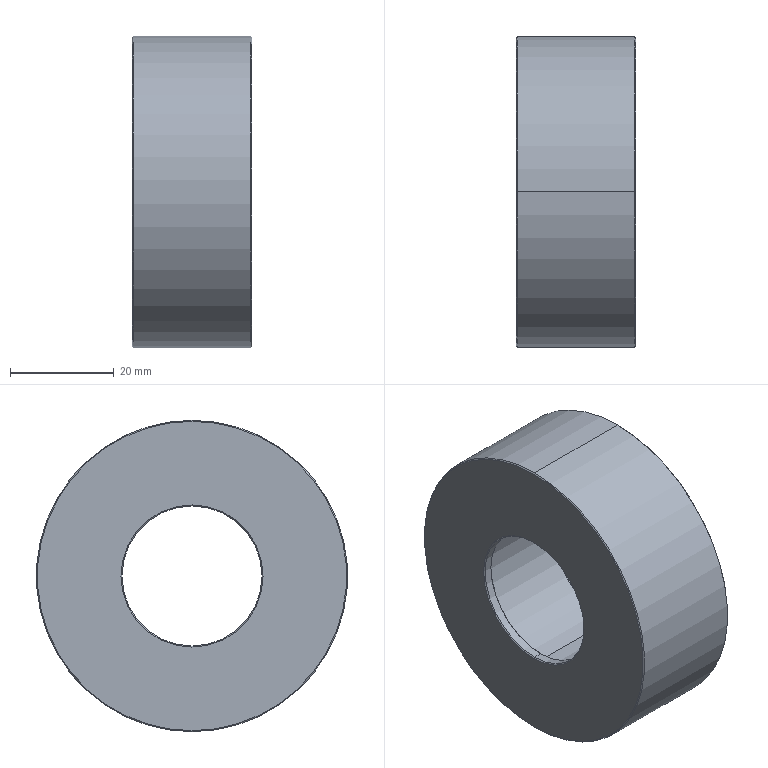Part | STEP file | Con lan ty | 1 solid | 25 faces | box 23 x 60 x 60 mm | volume 48906 mm3 | cone 10 | cylinder 10 | plane 5 | commonest cylinder face diameters 30 x4 27 x2 32.1 x2 60 x2
STEP:
#1=CARTESIAN_POINT('',(23.,0.,-29.8));
#2=VERTEX_POINT('',#1);
#3=CARTESIAN_POINT('',(23.,0.,29.8));
#4=VERTEX_POINT('',#3);
#5=CARTESIAN_POINT('',(23.,0.,0.));
#6=DIRECTION('',(1.,0.,0.));
#7=DIRECTION('',(0.,0.,1.));
#8=AXIS2_PLACEMENT_3D('',#5,#6,#7);
#9=CIRCLE('',#8,29.8);
#10=EDGE_CURVE('',#2,#4,#9,.T.);
#11=ORIENTED_EDGE('',*,*,#10,.F.);
#12=CARTESIAN_POINT('',(22.8,0.,-30.));
#13=VERTEX_POINT('',#12);
#14=CARTESIAN_POINT('',(22.8,0.,-30.));
#15=DIRECTION('',(-0.7071,0.,-0.7071));
#16=VECTOR('',#15,1000.);
#17=LINE('',#14,#16);
#18=EDGE_CURVE('',#2,#13,#17,.T.);
#19=ORIENTED_EDGE('',*,*,#18,.T.);
#20=CARTESIAN_POINT('',(22.8,0.,30.));
#21=VERTEX_POINT('',#20);
#22=CARTESIAN_POINT('',(22.8,0.,0.));
#23=DIRECTION('',(-1.,0.,0.));
#24=DIRECTION('',(0.,0.,1.));
#25=AXIS2_PLACEMENT_3D('',#22,#23,#24);
#26=CIRCLE('',#25,30.);
#27=EDGE_CURVE('',#21,#13,#26,.T.);
#28=ORIENTED_EDGE('',*,*,#27,.F.);
#29=CARTESIAN_POINT('',(22.8,0.,30.));
#30=DIRECTION('',(-0.7071,0.,0.7071));
#31=VECTOR('',#30,1000.);
#32=LINE('',#29,#31);
#33=EDGE_CURVE('',#4,#21,#32,.T.);
#34=ORIENTED_EDGE('',*,*,#33,.F.);
#35=EDGE_LOOP('',(#11,#19,#28,#34));
#36=FACE_OUTER_BOUND('',#35,.T.);
#37=CARTESIAN_POINT('',(22.8,0.,0.));
#38=DIRECTION('',(-1.,0.,0.));
#39=DIRECTION('',(0.,0.,1.));
#40=AXIS2_PLACEMENT_3D('',#37,#38,#39);
#41=CONICAL_SURFACE('',#40,30.,0.7854);
#42=ADVANCED_FACE('',(#36),#41,.T.);
#43=CARTESIAN_POINT('',(0.,0.,29.8));
#44=VERTEX_POINT('',#43);
#45=CARTESIAN_POINT('',(0.,0.,-29.8));
#46=VERTEX_POINT('',#45);
#47=CARTESIAN_POINT('',(0.,0.,0.));
#48=DIRECTION('',(-1.,0.,0.));
#49=DIRECTION('',(0.,0.,-1.));
#50=AXIS2_PLACEMENT_3D('',#47,#48,#49);
#51=CIRCLE('',#50,29.8);
#52=EDGE_CURVE('',#44,#46,#51,.T.);
#53=ORIENTED_EDGE('',*,*,#52,.F.);
#54=CARTESIAN_POINT('',(0.2,0.,30.));
#55=VERTEX_POINT('',#54);
#56=CARTESIAN_POINT('',(0.,0.,29.8));
#57=DIRECTION('',(0.7071,0.,0.7071));
#58=VECTOR('',#57,1000.);
#59=LINE('',#56,#58);
#60=EDGE_CURVE('',#44,#55,#59,.T.);
#61=ORIENTED_EDGE('',*,*,#60,.T.);
#62=CARTESIAN_POINT('',(0.2,0.,-30.));
#63=VERTEX_POINT('',#62);
#64=CARTESIAN_POINT('',(0.2,0.,0.));
#65=DIRECTION('',(1.,0.,0.));
#66=DIRECTION('',(0.,0.,-1.));
#67=AXIS2_PLACEMENT_3D('',#64,#65,#66);
#68=CIRCLE('',#67,30.);
#69=EDGE_CURVE('',#63,#55,#68,.T.);
#70=ORIENTED_EDGE('',*,*,#69,.F.);
#71=CARTESIAN_POINT('',(0.,0.,-29.8));
#72=DIRECTION('',(0.7071,0.,-0.7071));
#73=VECTOR('',#72,1000.);
#74=LINE('',#71,#73);
#75=EDGE_CURVE('',#46,#63,#74,.T.);
#76=ORIENTED_EDGE('',*,*,#75,.F.);
#77=EDGE_LOOP('',(#53,#61,#70,#76));
#78=FACE_OUTER_BOUND('',#77,.T.);
#79=CARTESIAN_POINT('',(0.,0.,0.));
#80=DIRECTION('',(1.,0.,0.));
#81=DIRECTION('',(0.,0.,-1.));
#82=AXIS2_PLACEMENT_3D('',#79,#80,#81);
#83=CONICAL_SURFACE('',#82,29.8,0.7854);
#84=ADVANCED_FACE('',(#78),#83,.T.);
#85=CARTESIAN_POINT('',(22.8,0.,15.));
#86=VERTEX_POINT('',#85);
#87=CARTESIAN_POINT('',(22.8,0.,-15.));
#88=VERTEX_POINT('',#87);
#89=CARTESIAN_POINT('',(22.8,0.,0.));
#90=DIRECTION('',(1.,0.,0.));
#91=DIRECTION('',(0.,0.,1.));
#92=AXIS2_PLACEMENT_3D('',#89,#90,#91);
#93=CIRCLE('',#92,15.);
#94=EDGE_CURVE('',#86,#88,#93,.T.);
#95=ORIENTED_EDGE('',*,*,#94,.F.);
#96=CARTESIAN_POINT('',(23.,0.,15.2));
#97=VERTEX_POINT('',#96);
#98=CARTESIAN_POINT('',(23.,0.,15.2));
#99=DIRECTION('',(0.7071,0.,0.7071));
#100=VECTOR('',#99,1000.);
#101=LINE('',#98,#100);
#102=EDGE_CURVE('',#86,#97,#101,.T.);
#103=ORIENTED_EDGE('',*,*,#102,.T.);
#104=CARTESIAN_POINT('',(23.,0.,-15.2));
#105=VERTEX_POINT('',#104);
#106=CARTESIAN_POINT('',(23.,0.,0.));
#107=DIRECTION('',(-1.,0.,0.));
#108=DIRECTION('',(0.,0.,1.));
#109=AXIS2_PLACEMENT_3D('',#106,#107,#108);
#110=CIRCLE('',#109,15.2);
#111=EDGE_CURVE('',#105,#97,#110,.T.);
#112=ORIENTED_EDGE('',*,*,#111,.F.);
#113=CARTESIAN_POINT('',(23.,0.,-15.2));
#114=DIRECTION('',(0.7071,0.,-0.7071));
#115=VECTOR('',#114,1000.);
#116=LINE('',#113,#115);
#117=EDGE_CURVE('',#88,#105,#116,.T.);
#118=ORIENTED_EDGE('',*,*,#117,.F.);
#119=EDGE_LOOP('',(#95,#103,#112,#118));
#120=FACE_OUTER_BOUND('',#119,.T.);
#121=CARTESIAN_POINT('',(23.,0.,0.));
#122=DIRECTION('',(1.,0.,0.));
#123=DIRECTION('',(0.,0.,-1.));
#124=AXIS2_PLACEMENT_3D('',#121,#122,#123);
#125=CONICAL_SURFACE('',#124,15.2,0.7854);
#126=ADVANCED_FACE('',(#120),#125,.F.);
#127=CARTESIAN_POINT('',(0.2,0.,-13.5));
#128=VERTEX_POINT('',#127);
#129=CARTESIAN_POINT('',(0.2,0.,13.5));
#130=VERTEX_POINT('',#129);
#131=CARTESIAN_POINT('',(0.2,0.,0.));
#132=DIRECTION('',(-1.,0.,0.));
#133=DIRECTION('',(0.,0.,-1.));
#134=AXIS2_PLACEMENT_3D('',#131,#132,#133);
#135=CIRCLE('',#134,13.5);
#136=EDGE_CURVE('',#128,#130,#135,.T.);
#137=ORIENTED_EDGE('',*,*,#136,.F.);
#138=CARTESIAN_POINT('',(0.,0.,-13.7));
#139=VERTEX_POINT('',#138);
#140=CARTESIAN_POINT('',(0.2,0.,-13.5));
#141=DIRECTION('',(-0.7071,0.,-0.7071));
#142=VECTOR('',#141,1000.);
#143=LINE('',#140,#142);
#144=EDGE_CURVE('',#128,#139,#143,.T.);
#145=ORIENTED_EDGE('',*,*,#144,.T.);
#146=CARTESIAN_POINT('',(0.,0.,13.7));
#147=VERTEX_POINT('',#146);
#148=CARTESIAN_POINT('',(0.,0.,0.));
#149=DIRECTION('',(1.,0.,0.));
#150=DIRECTION('',(0.,0.,-1.));
#151=AXIS2_PLACEMENT_3D('',#148,#149,#150);
#152=CIRCLE('',#151,13.7);
#153=EDGE_CURVE('',#147,#139,#152,.T.);
#154=ORIENTED_EDGE('',*,*,#153,.F.);
#155=CARTESIAN_POINT('',(0.2,0.,13.5));
#156=DIRECTION('',(-0.7071,0.,0.7071));
#157=VECTOR('',#156,1000.);
#158=LINE('',#155,#157);
#159=EDGE_CURVE('',#130,#147,#158,.T.);
#160=ORIENTED_EDGE('',*,*,#159,.F.);
#161=EDGE_LOOP('',(#137,#145,#154,#160));
#162=FACE_OUTER_BOUND('',#161,.T.);
#163=CARTESIAN_POINT('',(0.2,0.,0.));
#164=DIRECTION('',(-1.,0.,0.));
#165=DIRECTION('',(0.,0.,1.));
#166=AXIS2_PLACEMENT_3D('',#163,#164,#165);
#167=CONICAL_SURFACE('',#166,13.5,0.7854);
#168=ADVANCED_FACE('',(#162),#167,.F.);
#169=CARTESIAN_POINT('',(1.8,0.,13.5));
#170=VERTEX_POINT('',#169);
#171=CARTESIAN_POINT('',(1.8,0.,-13.5));
#172=VERTEX_POINT('',#171);
#173=CARTESIAN_POINT('',(1.8,0.,0.));
#174=DIRECTION('',(1.,0.,0.));
#175=DIRECTION('',(0.,0.,1.));
#176=AXIS2_PLACEMENT_3D('',#173,#174,#175);
#177=CIRCLE('',#176,13.5);
#178=EDGE_CURVE('',#170,#172,#177,.T.);
#179=ORIENTED_EDGE('',*,*,#178,.F.);
#180=CARTESIAN_POINT('',(2.,0.,13.7));
#181=VERTEX_POINT('',#180);
#182=CARTESIAN_POINT('',(2.,0.,13.7));
#183=DIRECTION('',(0.7071,0.,0.7071));
#184=VECTOR('',#183,1000.);
#185=LINE('',#182,#184);
#186=EDGE_CURVE('',#170,#181,#185,.T.);
#187=ORIENTED_EDGE('',*,*,#186,.T.);
#188=CARTESIAN_POINT('',(2.,0.,-13.7));
#189=VERTEX_POINT('',#188);
#190=CARTESIAN_POINT('',(2.,0.,0.));
#191=DIRECTION('',(-1.,0.,0.));
#192=DIRECTION('',(0.,0.,1.));
#193=AXIS2_PLACEMENT_3D('',#190,#191,#192);
#194=CIRCLE('',#193,13.7);
#195=EDGE_CURVE('',#189,#181,#194,.T.);
#196=ORIENTED_EDGE('',*,*,#195,.F.);
#197=CARTESIAN_POINT('',(2.,0.,-13.7));
#198=DIRECTION('',(0.7071,0.,-0.7071));
#199=VECTOR('',#198,1000.);
#200=LINE('',#197,#199);
#201=EDGE_CURVE('',#172,#189,#200,.T.);
#202=ORIENTED_EDGE('',*,*,#201,.F.);
#203=EDGE_LOOP('',(#179,#187,#196,#202));
#204=FACE_OUTER_BOUND('',#203,.T.);
#205=CARTESIAN_POINT('',(2.,0.,0.));
#206=DIRECTION('',(1.,0.,0.));
#207=DIRECTION('',(0.,0.,-1.));
#208=AXIS2_PLACEMENT_3D('',#205,#206,#207);
#209=CONICAL_SURFACE('',#208,13.7,0.7854);
#210=ADVANCED_FACE('',(#204),#209,.F.);
#211=ORIENTED_EDGE('',*,*,#27,.T.);
#212=CARTESIAN_POINT('',(0.,0.,-30.));
#213=DIRECTION('',(-1.,0.,0.));
#214=VECTOR('',#213,1000.);
#215=LINE('',#212,#214);
#216=EDGE_CURVE('',#13,#63,#215,.T.);
#217=ORIENTED_EDGE('',*,*,#216,.T.);
#218=ORIENTED_EDGE('',*,*,#69,.T.);
#219=CARTESIAN_POINT('',(0.,0.,30.));
#220=DIRECTION('',(-1.,0.,0.));
#221=VECTOR('',#220,1000.);
#222=LINE('',#219,#221);
#223=EDGE_CURVE('',#21,#55,#222,.T.);
#224=ORIENTED_EDGE('',*,*,#223,.F.);
#225=EDGE_LOOP('',(#211,#217,#218,#224));
#226=FACE_OUTER_BOUND('',#225,.T.);
#227=CARTESIAN_POINT('',(0.,0.,0.));
#228=DIRECTION('',(-1.,0.,0.));
#229=DIRECTION('',(0.,0.,1.));
#230=AXIS2_PLACEMENT_3D('',#227,#228,#229);
#231=CYLINDRICAL_SURFACE('',#230,30.);
#232=ADVANCED_FACE('',(#226),#231,.T.);
#233=ORIENTED_EDGE('',*,*,#94,.T.);
#234=CARTESIAN_POINT('',(21.2,0.,-15.));
#235=VERTEX_POINT('',#234);
#236=CARTESIAN_POINT('',(0.,0.,-15.));
#237=DIRECTION('',(-1.,0.,0.));
#238=VECTOR('',#237,1000.);
#239=LINE('',#236,#238);
#240=EDGE_CURVE('',#88,#235,#239,.T.);
#241=ORIENTED_EDGE('',*,*,#240,.T.);
#242=CARTESIAN_POINT('',(21.2,0.,15.));
#243=VERTEX_POINT('',#242);
#244=CARTESIAN_POINT('',(21.2,0.,0.));
#245=DIRECTION('',(-1.,0.,0.));
#246=DIRECTION('',(0.,0.,1.));
#247=AXIS2_PLACEMENT_3D('',#244,#245,#246);
#248=CIRCLE('',#247,15.);
#249=EDGE_CURVE('',#235,#243,#248,.T.);
#250=ORIENTED_EDGE('',*,*,#249,.T.);
#251=CARTESIAN_POINT('',(0.,0.,15.));
#252=DIRECTION('',(-1.,0.,0.));
#253=VECTOR('',#252,1000.);
#254=LINE('',#251,#253);
#255=EDGE_CURVE('',#86,#243,#254,.T.);
#256=ORIENTED_EDGE('',*,*,#255,.F.);
#257=EDGE_LOOP('',(#233,#241,#250,#256));
#258=FACE_OUTER_BOUND('',#257,.T.);
#259=CARTESIAN_POINT('',(0.,0.,0.));
#260=DIRECTION('',(-1.,0.,0.));
#261=DIRECTION('',(0.,0.,1.));
#262=AXIS2_PLACEMENT_3D('',#259,#260,#261);
#263=CYLINDRICAL_SURFACE('',#262,15.);
#264=ADVANCED_FACE('',(#258),#263,.F.);
#265=CARTESIAN_POINT('',(21.2,0.,-16.05));
#266=VERTEX_POINT('',#265);
#267=CARTESIAN_POINT('',(21.2,0.,16.05));
#268=VERTEX_POINT('',#267);
#269=CARTESIAN_POINT('',(21.2,0.,0.));
#270=DIRECTION('',(-1.,0.,0.));
#271=DIRECTION('',(0.,0.,1.));
#272=AXIS2_PLACEMENT_3D('',#269,#270,#271);
#273=CIRCLE('',#272,16.05);
#274=EDGE_CURVE('',#266,#268,#273,.T.);
#275=ORIENTED_EDGE('',*,*,#274,.F.);
#276=CARTESIAN_POINT('',(20.,0.,-16.05));
#277=VERTEX_POINT('',#276);
#278=CARTESIAN_POINT('',(0.,0.,-16.05));
#279=DIRECTION('',(-1.,0.,0.));
#280=VECTOR('',#279,1000.);
#281=LINE('',#278,#280);
#282=EDGE_CURVE('',#266,#277,#281,.T.);
#283=ORIENTED_EDGE('',*,*,#282,.T.);
#284=CARTESIAN_POINT('',(20.,0.,16.05));
#285=VERTEX_POINT('',#284);
#286=CARTESIAN_POINT('',(20.,0.,0.));
#287=DIRECTION('',(-1.,0.,0.));
#288=DIRECTION('',(0.,0.,1.));
#289=AXIS2_PLACEMENT_3D('',#286,#287,#288);
#290=CIRCLE('',#289,16.05);
#291=EDGE_CURVE('',#277,#285,#290,.T.);
#292=ORIENTED_EDGE('',*,*,#291,.T.);
#293=CARTESIAN_POINT('',(0.,0.,16.05));
#294=DIRECTION('',(-1.,0.,0.));
#295=VECTOR('',#294,1000.);
#296=LINE('',#293,#295);
#297=EDGE_CURVE('',#268,#285,#296,.T.);
#298=ORIENTED_EDGE('',*,*,#297,.F.);
#299=EDGE_LOOP('',(#275,#283,#292,#298));
#300=FACE_OUTER_BOUND('',#299,.T.);
#301=CARTESIAN_POINT('',(0.,0.,0.));
#302=DIRECTION('',(-1.,0.,0.));
#303=DIRECTION('',(0.,0.,1.));
#304=AXIS2_PLACEMENT_3D('',#301,#302,#303);
#305=CYLINDRICAL_SURFACE('',#304,16.05);
#306=ADVANCED_FACE('',(#300),#305,.F.);
#307=CARTESIAN_POINT('',(20.,0.,-15.));
#308=VERTEX_POINT('',#307);
#309=CARTESIAN_POINT('',(20.,0.,15.));
#310=VERTEX_POINT('',#309);
#311=CARTESIAN_POINT('',(20.,0.,0.));
#312=DIRECTION('',(-1.,0.,0.));
#313=DIRECTION('',(0.,0.,1.));
#314=AXIS2_PLACEMENT_3D('',#311,#312,#313);
#315=CIRCLE('',#314,15.);
#316=EDGE_CURVE('',#308,#310,#315,.T.);
#317=ORIENTED_EDGE('',*,*,#316,.F.);
#318=CARTESIAN_POINT('',(2.,0.,-15.));
#319=VERTEX_POINT('',#318);
#320=CARTESIAN_POINT('',(0.,0.,-15.));
#321=DIRECTION('',(-1.,0.,0.));
#322=VECTOR('',#321,1000.);
#323=LINE('',#320,#322);
#324=EDGE_CURVE('',#308,#319,#323,.T.);
#325=ORIENTED_EDGE('',*,*,#324,.T.);
#326=CARTESIAN_POINT('',(2.,0.,15.));
#327=VERTEX_POINT('',#326);
#328=CARTESIAN_POINT('',(2.,0.,0.));
#329=DIRECTION('',(-1.,0.,0.));
#330=DIRECTION('',(0.,0.,1.));
#331=AXIS2_PLACEMENT_3D('',#328,#329,#330);
#332=CIRCLE('',#331,15.);
#333=EDGE_CURVE('',#319,#327,#332,.T.);
#334=ORIENTED_EDGE('',*,*,#333,.T.);
#335=CARTESIAN_POINT('',(0.,0.,15.));
#336=DIRECTION('',(-1.,0.,0.));
#337=VECTOR('',#336,1000.);
#338=LINE('',#335,#337);
#339=EDGE_CURVE('',#310,#327,#338,.T.);
#340=ORIENTED_EDGE('',*,*,#339,.F.);
#341=EDGE_LOOP('',(#317,#325,#334,#340));
#342=FACE_OUTER_BOUND('',#341,.T.);
#343=CARTESIAN_POINT('',(0.,0.,0.));
#344=DIRECTION('',(-1.,0.,0.));
#345=DIRECTION('',(0.,0.,1.));
#346=AXIS2_PLACEMENT_3D('',#343,#344,#345);
#347=CYLINDRICAL_SURFACE('',#346,15.);
#348=ADVANCED_FACE('',(#342),#347,.F.);
#349=ORIENTED_EDGE('',*,*,#178,.T.);
#350=CARTESIAN_POINT('',(0.,0.,-13.5));
#351=DIRECTION('',(-1.,0.,0.));
#352=VECTOR('',#351,1000.);
#353=LINE('',#350,#352);
#354=EDGE_CURVE('',#172,#128,#353,.T.);
#355=ORIENTED_EDGE('',*,*,#354,.T.);
#356=ORIENTED_EDGE('',*,*,#136,.T.);
#357=CARTESIAN_POINT('',(0.,0.,13.5));
#358=DIRECTION('',(-1.,0.,0.));
#359=VECTOR('',#358,1000.);
#360=LINE('',#357,#359);
#361=EDGE_CURVE('',#170,#130,#360,.T.);
#362=ORIENTED_EDGE('',*,*,#361,.F.);
#363=EDGE_LOOP('',(#349,#355,#356,#362));
#364=FACE_OUTER_BOUND('',#363,.T.);
#365=CARTESIAN_POINT('',(0.,0.,0.));
#366=DIRECTION('',(-1.,0.,0.));
#367=DIRECTION('',(0.,0.,1.));
#368=AXIS2_PLACEMENT_3D('',#365,#366,#367);
#369=CYLINDRICAL_SURFACE('',#368,13.5);
#370=ADVANCED_FACE('',(#364),#369,.F.);
#371=ORIENTED_EDGE('',*,*,#153,.T.);
#372=CARTESIAN_POINT('',(0.,0.,0.));
#373=DIRECTION('',(1.,0.,0.));
#374=DIRECTION('',(0.,0.,-1.));
#375=AXIS2_PLACEMENT_3D('',#372,#373,#374);
#376=CIRCLE('',#375,13.7);
#377=EDGE_CURVE('',#139,#147,#376,.T.);
#378=ORIENTED_EDGE('',*,*,#377,.T.);
#379=EDGE_LOOP('',(#371,#378));
#380=FACE_BOUND('',#379,.T.);
#381=CARTESIAN_POINT('',(0.,0.,0.));
#382=DIRECTION('',(-1.,0.,0.));
#383=DIRECTION('',(0.,0.,-1.));
#384=AXIS2_PLACEMENT_3D('',#381,#382,#383);
#385=CIRCLE('',#384,29.8);
#386=EDGE_CURVE('',#46,#44,#385,.T.);
#387=ORIENTED_EDGE('',*,*,#386,.T.);
#388=ORIENTED_EDGE('',*,*,#52,.T.);
#389=EDGE_LOOP('',(#387,#388));
#390=FACE_OUTER_BOUND('',#389,.T.);
#391=CARTESIAN_POINT('',(0.,30.,0.));
#392=DIRECTION('',(1.,0.,0.));
#393=DIRECTION('',(0.,0.,-1.));
#394=AXIS2_PLACEMENT_3D('',#391,#392,#393);
#395=PLANE('',#394);
#396=ADVANCED_FACE('',(#380,#390),#395,.F.);
#397=ORIENTED_EDGE('',*,*,#354,.F.);
#398=CARTESIAN_POINT('',(1.8,0.,0.));
#399=DIRECTION('',(1.,0.,0.));
#400=DIRECTION('',(0.,0.,1.));
#401=AXIS2_PLACEMENT_3D('',#398,#399,#400);
#402=CIRCLE('',#401,13.5);
#403=EDGE_CURVE('',#172,#170,#402,.T.);
#404=ORIENTED_EDGE('',*,*,#403,.T.);
#405=ORIENTED_EDGE('',*,*,#361,.T.);
#406=CARTESIAN_POINT('',(0.2,0.,0.));
#407=DIRECTION('',(-1.,0.,0.));
#408=DIRECTION('',(0.,0.,-1.));
#409=AXIS2_PLACEMENT_3D('',#406,#407,#408);
#410=CIRCLE('',#409,13.5);
#411=EDGE_CURVE('',#130,#128,#410,.T.);
#412=ORIENTED_EDGE('',*,*,#411,.T.);
#413=EDGE_LOOP('',(#397,#404,#405,#412));
#414=FACE_OUTER_BOUND('',#413,.T.);
#415=CARTESIAN_POINT('',(0.,0.,0.));
#416=DIRECTION('',(-1.,0.,0.));
#417=DIRECTION('',(0.,0.,1.));
#418=AXIS2_PLACEMENT_3D('',#415,#416,#417);
#419=CYLINDRICAL_SURFACE('',#418,13.5);
#420=ADVANCED_FACE('',(#414),#419,.F.);
#421=ORIENTED_EDGE('',*,*,#195,.T.);
#422=CARTESIAN_POINT('',(2.,0.,0.));
#423=DIRECTION('',(-1.,0.,0.));
#424=DIRECTION('',(0.,0.,1.));
#425=AXIS2_PLACEMENT_3D('',#422,#423,#424);
#426=CIRCLE('',#425,13.7);
#427=EDGE_CURVE('',#181,#189,#426,.T.);
#428=ORIENTED_EDGE('',*,*,#427,.T.);
#429=EDGE_LOOP('',(#421,#428));
#430=FACE_BOUND('',#429,.T.);
#431=CARTESIAN_POINT('',(2.,0.,0.));
#432=DIRECTION('',(-1.,0.,0.));
#433=DIRECTION('',(0.,0.,1.));
#434=AXIS2_PLACEMENT_3D('',#431,#432,#433);
#435=CIRCLE('',#434,15.);
#436=EDGE_CURVE('',#327,#319,#435,.T.);
#437=ORIENTED_EDGE('',*,*,#436,.F.);
#438=ORIENTED_EDGE('',*,*,#333,.F.);
#439=EDGE_LOOP('',(#437,#438));
#440=FACE_OUTER_BOUND('',#439,.T.);
#441=CARTESIAN_POINT('',(2.,13.5,0.));
#442=DIRECTION('',(-1.,0.,0.));
#443=DIRECTION('',(0.,0.,1.));
#444=AXIS2_PLACEMENT_3D('',#441,#442,#443);
#445=PLANE('',#444);
#446=ADVANCED_FACE('',(#430,#440),#445,.F.);
#447=ORIENTED_EDGE('',*,*,#324,.F.);
#448=CARTESIAN_POINT('',(20.,0.,0.));
#449=DIRECTION('',(-1.,0.,0.));
#450=DIRECTION('',(0.,0.,1.));
#451=AXIS2_PLACEMENT_3D('',#448,#449,#450);
#452=CIRCLE('',#451,15.);
#453=EDGE_CURVE('',#310,#308,#452,.T.);
#454=ORIENTED_EDGE('',*,*,#453,.F.);
#455=ORIENTED_EDGE('',*,*,#339,.T.);
#456=ORIENTED_EDGE('',*,*,#436,.T.);
#457=EDGE_LOOP('',(#447,#454,#455,#456));
#458=FACE_OUTER_BOUND('',#457,.T.);
#459=CARTESIAN_POINT('',(0.,0.,0.));
#460=DIRECTION('',(-1.,0.,0.));
#461=DIRECTION('',(0.,0.,1.));
#462=AXIS2_PLACEMENT_3D('',#459,#460,#461);
#463=CYLINDRICAL_SURFACE('',#462,15.);
#464=ADVANCED_FACE('',(#458),#463,.F.);
#465=CARTESIAN_POINT('',(20.,0.,0.));
#466=DIRECTION('',(-1.,0.,0.));
#467=DIRECTION('',(0.,0.,1.));
#468=AXIS2_PLACEMENT_3D('',#465,#466,#467);
#469=CIRCLE('',#468,16.05);
#470=EDGE_CURVE('',#285,#277,#469,.T.);
#471=ORIENTED_EDGE('',*,*,#470,.F.);
#472=ORIENTED_EDGE('',*,*,#291,.F.);
#473=EDGE_LOOP('',(#471,#472));
#474=FACE_OUTER_BOUND('',#473,.T.);
#475=ORIENTED_EDGE('',*,*,#453,.T.);
#476=ORIENTED_EDGE('',*,*,#316,.T.);
#477=EDGE_LOOP('',(#475,#476));
#478=FACE_BOUND('',#477,.T.);
#479=CARTESIAN_POINT('',(20.,16.05,0.));
#480=DIRECTION('',(-1.,0.,0.));
#481=DIRECTION('',(0.,0.,1.));
#482=AXIS2_PLACEMENT_3D('',#479,#480,#481);
#483=PLANE('',#482);
#484=ADVANCED_FACE('',(#474,#478),#483,.F.);
#485=ORIENTED_EDGE('',*,*,#282,.F.);
#486=CARTESIAN_POINT('',(21.2,0.,0.));
#487=DIRECTION('',(-1.,0.,0.));
#488=DIRECTION('',(0.,0.,1.));
#489=AXIS2_PLACEMENT_3D('',#486,#487,#488);
#490=CIRCLE('',#489,16.05);
#491=EDGE_CURVE('',#268,#266,#490,.T.);
#492=ORIENTED_EDGE('',*,*,#491,.F.);
#493=ORIENTED_EDGE('',*,*,#297,.T.);
#494=ORIENTED_EDGE('',*,*,#470,.T.);
#495=EDGE_LOOP('',(#485,#492,#493,#494));
#496=FACE_OUTER_BOUND('',#495,.T.);
#497=CARTESIAN_POINT('',(0.,0.,0.));
#498=DIRECTION('',(-1.,0.,0.));
#499=DIRECTION('',(0.,0.,1.));
#500=AXIS2_PLACEMENT_3D('',#497,#498,#499);
#501=CYLINDRICAL_SURFACE('',#500,16.05);
#502=ADVANCED_FACE('',(#496),#501,.F.);
#503=CARTESIAN_POINT('',(21.2,0.,0.));
#504=DIRECTION('',(-1.,0.,0.));
#505=DIRECTION('',(0.,0.,1.));
#506=AXIS2_PLACEMENT_3D('',#503,#504,#505);
#507=CIRCLE('',#506,15.);
#508=EDGE_CURVE('',#243,#235,#507,.T.);
#509=ORIENTED_EDGE('',*,*,#508,.F.);
#510=ORIENTED_EDGE('',*,*,#249,.F.);
#511=EDGE_LOOP('',(#509,#510));
#512=FACE_BOUND('',#511,.T.);
#513=ORIENTED_EDGE('',*,*,#491,.T.);
#514=ORIENTED_EDGE('',*,*,#274,.T.);
#515=EDGE_LOOP('',(#513,#514));
#516=FACE_OUTER_BOUND('',#515,.T.);
#517=CARTESIAN_POINT('',(21.2,15.,0.));
#518=DIRECTION('',(1.,0.,0.));
#519=DIRECTION('',(0.,0.,-1.));
#520=AXIS2_PLACEMENT_3D('',#517,#518,#519);
#521=PLANE('',#520);
#522=ADVANCED_FACE('',(#512,#516),#521,.F.);
#523=ORIENTED_EDGE('',*,*,#240,.F.);
#524=CARTESIAN_POINT('',(22.8,0.,0.));
#525=DIRECTION('',(1.,0.,0.));
#526=DIRECTION('',(0.,0.,1.));
#527=AXIS2_PLACEMENT_3D('',#524,#525,#526);
#528=CIRCLE('',#527,15.);
#529=EDGE_CURVE('',#88,#86,#528,.T.);
#530=ORIENTED_EDGE('',*,*,#529,.T.);
#531=ORIENTED_EDGE('',*,*,#255,.T.);
#532=ORIENTED_EDGE('',*,*,#508,.T.);
#533=EDGE_LOOP('',(#523,#530,#531,#532));
#534=FACE_OUTER_BOUND('',#533,.T.);
#535=CARTESIAN_POINT('',(0.,0.,0.));
#536=DIRECTION('',(-1.,0.,0.));
#537=DIRECTION('',(0.,0.,1.));
#538=AXIS2_PLACEMENT_3D('',#535,#536,#537);
#539=CYLINDRICAL_SURFACE('',#538,15.);
#540=ADVANCED_FACE('',(#534),#539,.F.);
#541=ORIENTED_EDGE('',*,*,#111,.T.);
#542=CARTESIAN_POINT('',(23.,0.,0.));
#543=DIRECTION('',(-1.,0.,0.));
#544=DIRECTION('',(0.,0.,1.));
#545=AXIS2_PLACEMENT_3D('',#542,#543,#544);
#546=CIRCLE('',#545,15.2);
#547=EDGE_CURVE('',#97,#105,#546,.T.);
#548=ORIENTED_EDGE('',*,*,#547,.T.);
#549=EDGE_LOOP('',(#541,#548));
#550=FACE_BOUND('',#549,.T.);
#551=CARTESIAN_POINT('',(23.,0.,0.));
#552=DIRECTION('',(1.,0.,0.));
#553=DIRECTION('',(0.,0.,1.));
#554=AXIS2_PLACEMENT_3D('',#551,#552,#553);
#555=CIRCLE('',#554,29.8);
#556=EDGE_CURVE('',#4,#2,#555,.T.);
#557=ORIENTED_EDGE('',*,*,#556,.T.);
#558=ORIENTED_EDGE('',*,*,#10,.T.);
#559=EDGE_LOOP('',(#557,#558));
#560=FACE_OUTER_BOUND('',#559,.T.);
#561=CARTESIAN_POINT('',(23.,15.,0.));
#562=DIRECTION('',(-1.,0.,0.));
#563=DIRECTION('',(0.,0.,1.));
#564=AXIS2_PLACEMENT_3D('',#561,#562,#563);
#565=PLANE('',#564);
#566=ADVANCED_FACE('',(#550,#560),#565,.F.);
#567=ORIENTED_EDGE('',*,*,#216,.F.);
#568=CARTESIAN_POINT('',(22.8,0.,0.));
#569=DIRECTION('',(-1.,0.,0.));
#570=DIRECTION('',(0.,0.,1.));
#571=AXIS2_PLACEMENT_3D('',#568,#569,#570);
#572=CIRCLE('',#571,30.);
#573=EDGE_CURVE('',#13,#21,#572,.T.);
#574=ORIENTED_EDGE('',*,*,#573,.T.);
#575=ORIENTED_EDGE('',*,*,#223,.T.);
#576=CARTESIAN_POINT('',(0.2,0.,0.));
#577=DIRECTION('',(1.,0.,0.));
#578=DIRECTION('',(0.,0.,-1.));
#579=AXIS2_PLACEMENT_3D('',#576,#577,#578);
#580=CIRCLE('',#579,30.);
#581=EDGE_CURVE('',#55,#63,#580,.T.);
#582=ORIENTED_EDGE('',*,*,#581,.T.);
#583=EDGE_LOOP('',(#567,#574,#575,#582));
#584=FACE_OUTER_BOUND('',#583,.T.);
#585=CARTESIAN_POINT('',(0.,0.,0.));
#586=DIRECTION('',(-1.,0.,0.));
#587=DIRECTION('',(0.,0.,1.));
#588=AXIS2_PLACEMENT_3D('',#585,#586,#587);
#589=CYLINDRICAL_SURFACE('',#588,30.);
#590=ADVANCED_FACE('',(#584),#589,.T.);
#591=ORIENTED_EDGE('',*,*,#186,.F.);
#592=ORIENTED_EDGE('',*,*,#403,.F.);
#593=ORIENTED_EDGE('',*,*,#201,.T.);
#594=ORIENTED_EDGE('',*,*,#427,.F.);
#595=EDGE_LOOP('',(#591,#592,#593,#594));
#596=FACE_OUTER_BOUND('',#595,.T.);
#597=CARTESIAN_POINT('',(2.,0.,0.));
#598=DIRECTION('',(1.,0.,0.));
#599=DIRECTION('',(0.,0.,-1.));
#600=AXIS2_PLACEMENT_3D('',#597,#598,#599);
#601=CONICAL_SURFACE('',#600,13.7,0.7854);
#602=ADVANCED_FACE('',(#596),#601,.F.);
#603=ORIENTED_EDGE('',*,*,#144,.F.);
#604=ORIENTED_EDGE('',*,*,#411,.F.);
#605=ORIENTED_EDGE('',*,*,#159,.T.);
#606=ORIENTED_EDGE('',*,*,#377,.F.);
#607=EDGE_LOOP('',(#603,#604,#605,#606));
#608=FACE_OUTER_BOUND('',#607,.T.);
#609=CARTESIAN_POINT('',(0.2,0.,0.));
#610=DIRECTION('',(-1.,0.,0.));
#611=DIRECTION('',(0.,0.,1.));
#612=AXIS2_PLACEMENT_3D('',#609,#610,#611);
#613=CONICAL_SURFACE('',#612,13.5,0.7854);
#614=ADVANCED_FACE('',(#608),#613,.F.);
#615=ORIENTED_EDGE('',*,*,#102,.F.);
#616=ORIENTED_EDGE('',*,*,#529,.F.);
#617=ORIENTED_EDGE('',*,*,#117,.T.);
#618=ORIENTED_EDGE('',*,*,#547,.F.);
#619=EDGE_LOOP('',(#615,#616,#617,#618));
#620=FACE_OUTER_BOUND('',#619,.T.);
#621=CARTESIAN_POINT('',(23.,0.,0.));
#622=DIRECTION('',(1.,0.,0.));
#623=DIRECTION('',(0.,0.,-1.));
#624=AXIS2_PLACEMENT_3D('',#621,#622,#623);
#625=CONICAL_SURFACE('',#624,15.2,0.7854);
#626=ADVANCED_FACE('',(#620),#625,.F.);
#627=ORIENTED_EDGE('',*,*,#60,.F.);
#628=ORIENTED_EDGE('',*,*,#386,.F.);
#629=ORIENTED_EDGE('',*,*,#75,.T.);
#630=ORIENTED_EDGE('',*,*,#581,.F.);
#631=EDGE_LOOP('',(#627,#628,#629,#630));
#632=FACE_OUTER_BOUND('',#631,.T.);
#633=CARTESIAN_POINT('',(0.,0.,0.));
#634=DIRECTION('',(1.,0.,0.));
#635=DIRECTION('',(0.,0.,-1.));
#636=AXIS2_PLACEMENT_3D('',#633,#634,#635);
#637=CONICAL_SURFACE('',#636,29.8,0.7854);
#638=ADVANCED_FACE('',(#632),#637,.T.);
#639=ORIENTED_EDGE('',*,*,#18,.F.);
#640=ORIENTED_EDGE('',*,*,#556,.F.);
#641=ORIENTED_EDGE('',*,*,#33,.T.);
#642=ORIENTED_EDGE('',*,*,#573,.F.);
#643=EDGE_LOOP('',(#639,#640,#641,#642));
#644=FACE_OUTER_BOUND('',#643,.T.);
#645=CARTESIAN_POINT('',(22.8,0.,0.));
#646=DIRECTION('',(-1.,0.,0.));
#647=DIRECTION('',(0.,0.,1.));
#648=AXIS2_PLACEMENT_3D('',#645,#646,#647);
#649=CONICAL_SURFACE('',#648,30.,0.7854);
#650=ADVANCED_FACE('',(#644),#649,.T.);
#651=CLOSED_SHELL('',(#42,#84,#126,#168,#210,#232,#264,#306,#348,#370,#396,#420,#446,#464,#484,#502,#522,#540,#566,#590,#602,#614,#626,#638,#650));
#652=MANIFOLD_SOLID_BREP('',#651);
#653=CARTESIAN_POINT('',(0.,0.,0.));
#654=DIRECTION('',(0.,0.,1.));
#655=DIRECTION('',(1.,0.,0.));
#656=AXIS2_PLACEMENT_3D('',#653,#654,#655);
#657=(LENGTH_UNIT()NAMED_UNIT(*)SI_UNIT(.MILLI.,.METRE.));
#658=UNCERTAINTY_MEASURE_WITH_UNIT(LENGTH_MEASURE(0.00001),#657,'','');
#659=(NAMED_UNIT(*)PLANE_ANGLE_UNIT()SI_UNIT($,.RADIAN.));
#660=(NAMED_UNIT(*)SI_UNIT($,.STERADIAN.)SOLID_ANGLE_UNIT());
#661=(GEOMETRIC_REPRESENTATION_CONTEXT(3)GLOBAL_UNCERTAINTY_ASSIGNED_CONTEXT((#658))GLOBAL_UNIT_ASSIGNED_CONTEXT((#657,#659,#660))REPRESENTATION_CONTEXT('',''));
#662=ADVANCED_BREP_SHAPE_REPRESENTATION('',(#652,#656),#661);